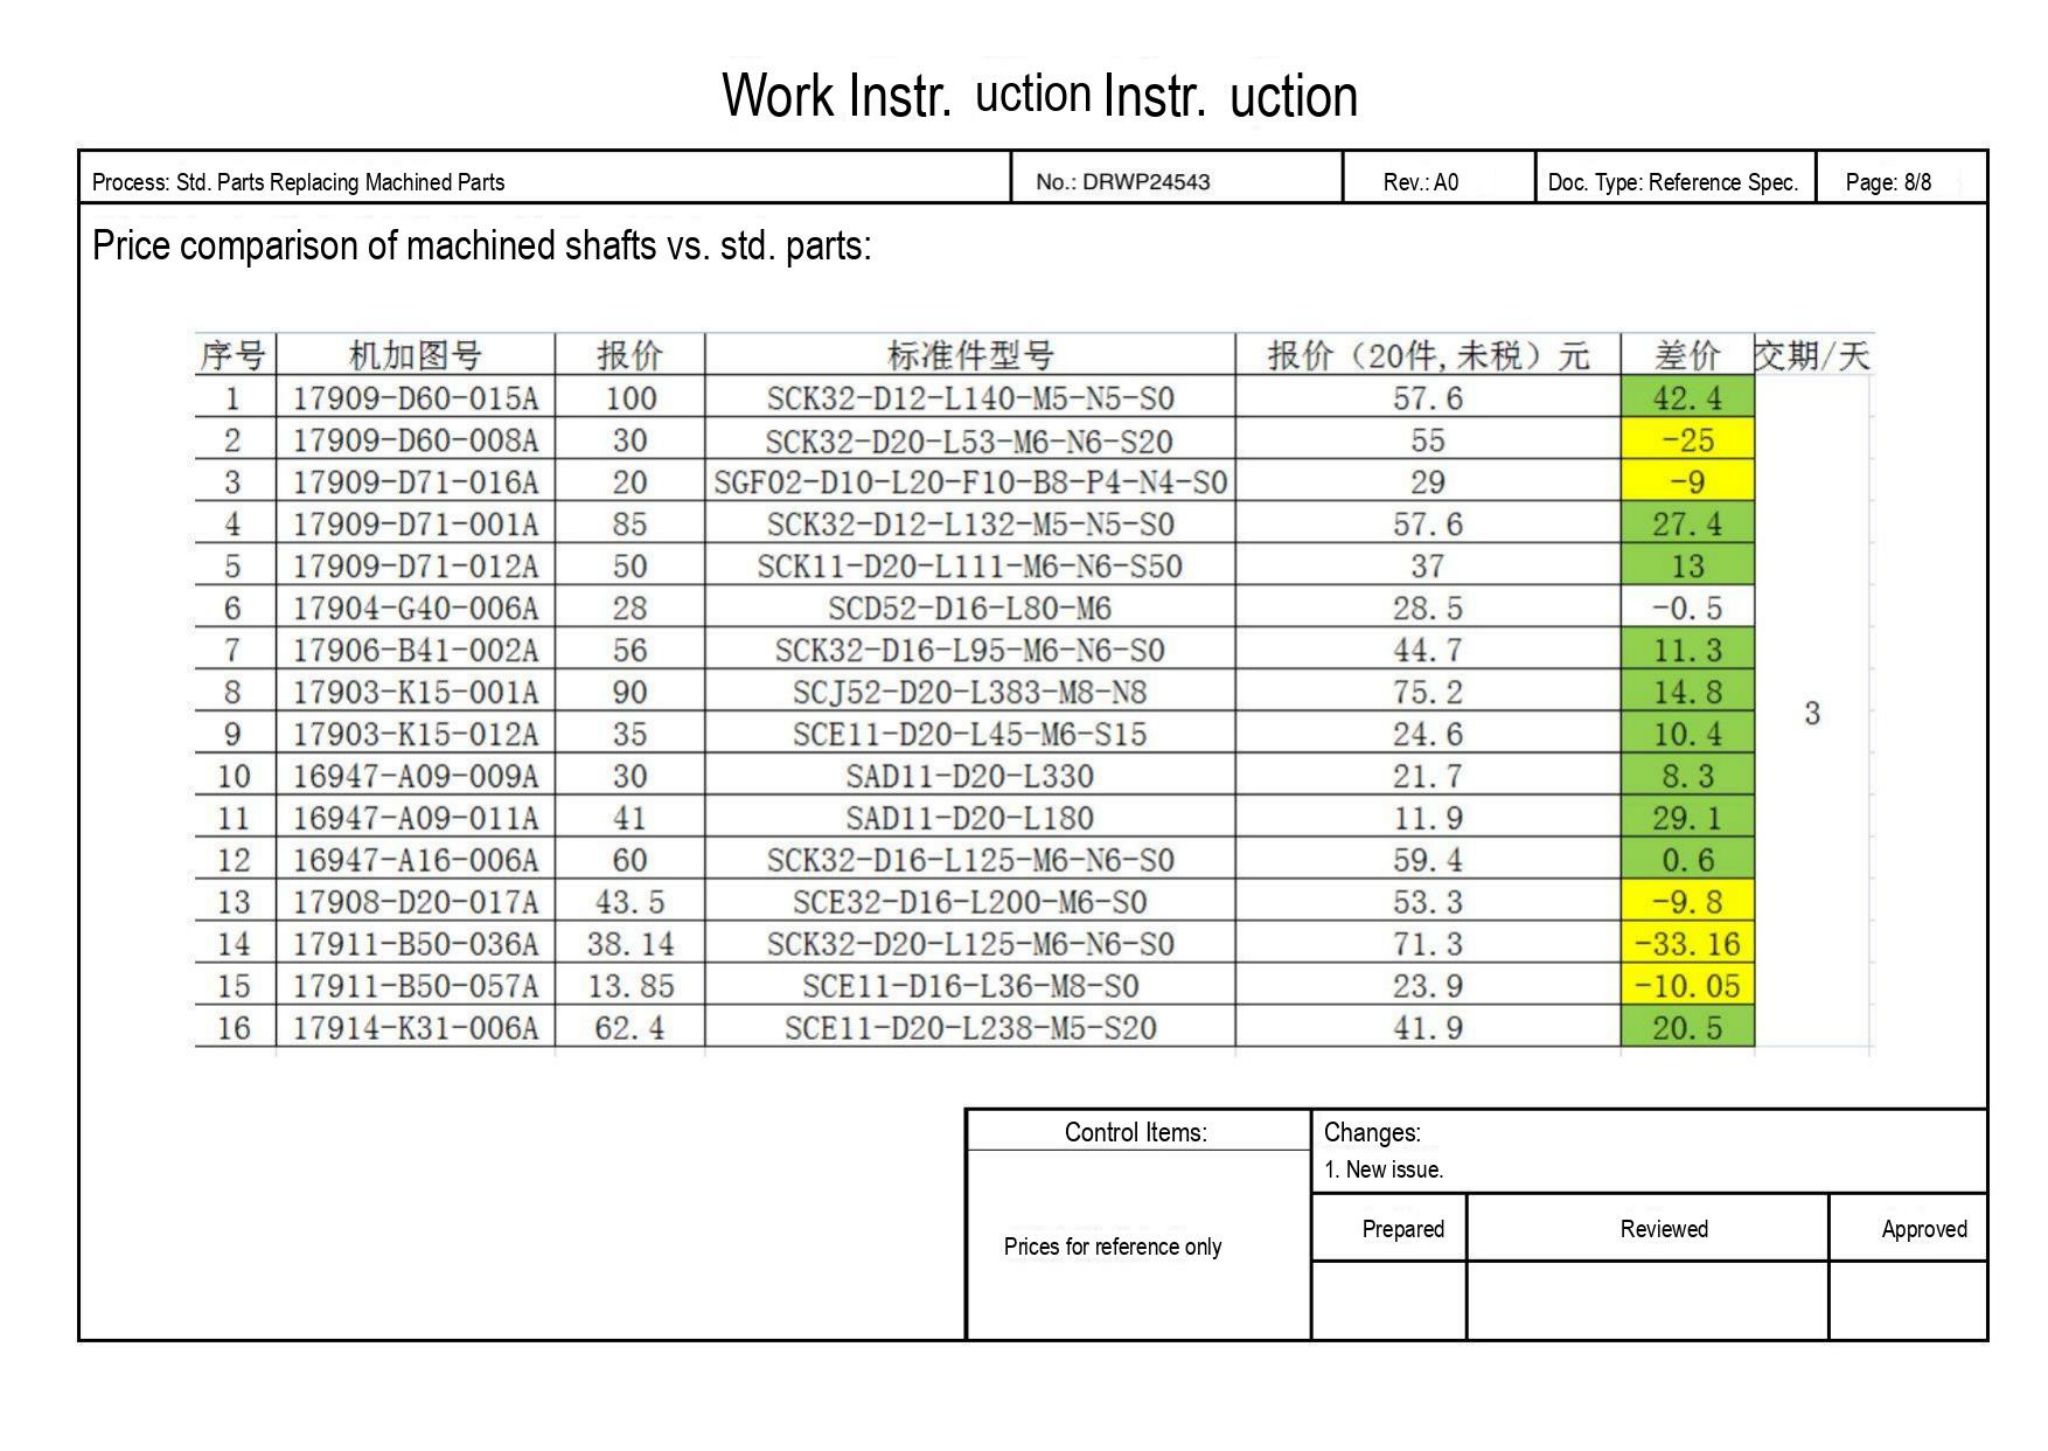Work Instr. uction Instr. uction

| Process: Std. Parts Replacing Machined Parts | No.: DRWP24543 | Rev.: A0 | Doc. Type: Reference Spec. | Page: 8/8 |
|---|---|---|---|---|

Price comparison of machined shafts vs. std. parts:

| 序号 | 机加图号 | 报价 | 标准件型号 | 报价（20件，未税）元 | 差价 | 交期/天 |
|---|---|---|---|---|---|---|
| 1 | 17909-D60-015A | 100 | SCK32-D12-L140-M5-N5-S0 | 57.6 | 42.4 | 3 |
| 2 | 17909-D60-008A | 30 | SCK32-D20-L53-M6-N6-S20 | 55 | -25 | |
| 3 | 17909-D71-016A | 20 | SGF02-D10-L20-F10-B8-P4-N4-S0 | 29 | -9 | |
| 4 | 17909-D71-001A | 85 | SCK32-D12-L132-M5-N5-S0 | 57.6 | 27.4 | |
| 5 | 17909-D71-012A | 50 | SCK11-D20-L111-M6-N6-S50 | 37 | 13 | |
| 6 | 17904-G40-006A | 28 | SCD52-D16-L80-M6 | 28.5 | -0.5 | |
| 7 | 17906-B41-002A | 56 | SCK32-D16-L95-M6-N6-S0 | 44.7 | 11.3 | |
| 8 | 17903-K15-001A | 90 | SCJ52-D20-L383-M8-N8 | 75.2 | 14.8 | |
| 9 | 17903-K15-012A | 35 | SCE11-D20-L45-M6-S15 | 24.6 | 10.4 | |
| 10 | 16947-A09-009A | 30 | SAD11-D20-L330 | 21.7 | 8.3 | |
| 11 | 16947-A09-011A | 41 | SAD11-D20-L180 | 11.9 | 29.1 | |
| 12 | 16947-A16-006A | 60 | SCK32-D16-L125-M6-N6-S0 | 59.4 | 0.6 | |
| 13 | 17908-D20-017A | 43.5 | SCE32-D16-L200-M6-S0 | 53.3 | -9.8 | |
| 14 | 17911-B50-036A | 38.14 | SCK32-D20-L125-M6-N6-S0 | 71.3 | -33.16 | |
| 15 | 17911-B50-057A | 13.85 | SCE11-D16-L36-M8-S0 | 23.9 | -10.05 | |
| 16 | 17914-K31-006A | 62.4 | SCE11-D20-L238-M5-S20 | 41.9 | 20.5 | |

| Control Items: | Changes: 1. New issue. | | |
|---|---|---|---|
| Prices for reference only | Prepared | Reviewed | Approved |
| | | | |